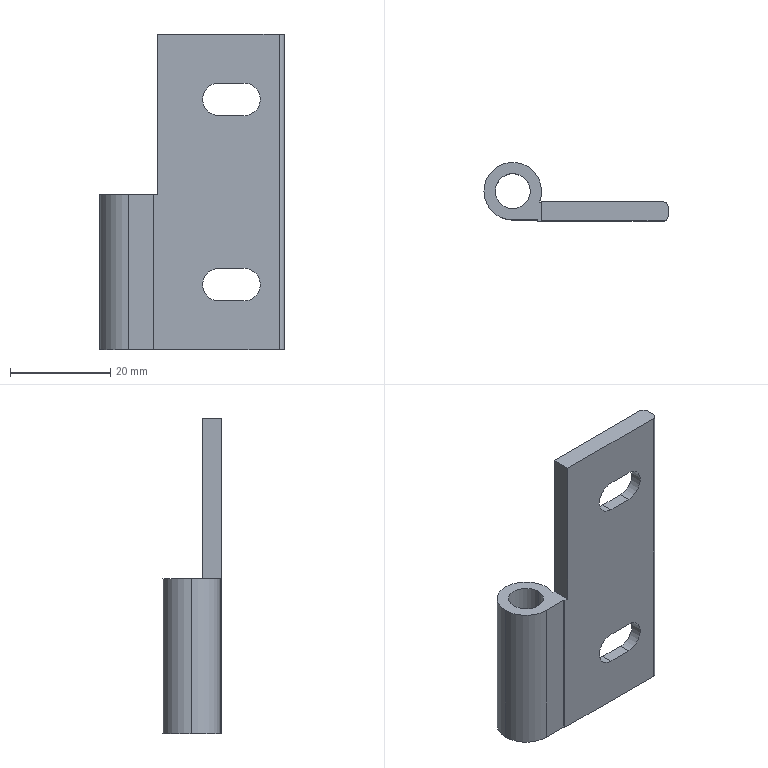Part | NX | features BREP 1 | 1 solid | 38 faces | box 36.75 x 11.75 x 63 mm | volume 7508 mm3 | cylinder 19 | plane 19 | commonest cylinder face diameters 6.5 x6 11 x6 11.5 x3 2 x2 7 x2
STEP:
#1=CARTESIAN_POINT('',(12.5,-3.7,18.5));
#2=VERTEX_POINT('',#1);
#3=CARTESIAN_POINT('',(18.,-3.7,24.));
#4=VERTEX_POINT('',#3);
#5=CARTESIAN_POINT('',(18.,-3.7,18.5));
#6=DIRECTION('',(0.,1.,0.));
#7=DIRECTION('',(-1.,0.,0.));
#8=AXIS2_PLACEMENT_3D('',#5,#6,#7);
#9=CIRCLE('',#8,5.5);
#10=EDGE_CURVE('',#2,#4,#9,.T.);
#11=ORIENTED_EDGE('',*,*,#10,.F.);
#12=CARTESIAN_POINT('',(12.5,-2.2,18.5));
#13=VERTEX_POINT('',#12);
#14=CARTESIAN_POINT('',(12.5,-3.7,18.5));
#15=DIRECTION('',(0.,1.,0.));
#16=VECTOR('',#15,1000.);
#17=LINE('',#14,#16);
#18=EDGE_CURVE('',#2,#13,#17,.T.);
#19=ORIENTED_EDGE('',*,*,#18,.T.);
#20=CARTESIAN_POINT('',(18.,-2.2,24.));
#21=VERTEX_POINT('',#20);
#22=CARTESIAN_POINT('',(18.,-2.2,18.5));
#23=DIRECTION('',(0.,1.,0.));
#24=DIRECTION('',(-1.,0.,0.));
#25=AXIS2_PLACEMENT_3D('',#22,#23,#24);
#26=CIRCLE('',#25,5.5);
#27=EDGE_CURVE('',#13,#21,#26,.T.);
#28=ORIENTED_EDGE('',*,*,#27,.T.);
#29=CARTESIAN_POINT('',(18.,-3.7,24.));
#30=DIRECTION('',(0.,1.,0.));
#31=VECTOR('',#30,1000.);
#32=LINE('',#29,#31);
#33=EDGE_CURVE('',#4,#21,#32,.T.);
#34=ORIENTED_EDGE('',*,*,#33,.F.);
#35=EDGE_LOOP('',(#11,#19,#28,#34));
#36=FACE_BOUND('',#35,.T.);
#37=CARTESIAN_POINT('',(18.,-3.7,18.5));
#38=DIRECTION('',(0.,1.,0.));
#39=DIRECTION('',(-1.,0.,0.));
#40=AXIS2_PLACEMENT_3D('',#37,#38,#39);
#41=CYLINDRICAL_SURFACE('',#40,5.5);
#42=ADVANCED_FACE('',(#36),#41,.F.);
#43=CARTESIAN_POINT('',(12.5,-3.7,-18.5));
#44=VERTEX_POINT('',#43);
#45=CARTESIAN_POINT('',(18.,-3.7,-13.));
#46=VERTEX_POINT('',#45);
#47=CARTESIAN_POINT('',(18.,-3.7,-18.5));
#48=DIRECTION('',(0.,1.,0.));
#49=DIRECTION('',(-1.,0.,0.));
#50=AXIS2_PLACEMENT_3D('',#47,#48,#49);
#51=CIRCLE('',#50,5.5);
#52=EDGE_CURVE('',#44,#46,#51,.T.);
#53=ORIENTED_EDGE('',*,*,#52,.F.);
#54=CARTESIAN_POINT('',(12.5,-2.2,-18.5));
#55=VERTEX_POINT('',#54);
#56=CARTESIAN_POINT('',(12.5,-3.7,-18.5));
#57=DIRECTION('',(0.,1.,0.));
#58=VECTOR('',#57,1000.);
#59=LINE('',#56,#58);
#60=EDGE_CURVE('',#44,#55,#59,.T.);
#61=ORIENTED_EDGE('',*,*,#60,.T.);
#62=CARTESIAN_POINT('',(18.,-2.2,-13.));
#63=VERTEX_POINT('',#62);
#64=CARTESIAN_POINT('',(18.,-2.2,-18.5));
#65=DIRECTION('',(0.,1.,0.));
#66=DIRECTION('',(-1.,0.,0.));
#67=AXIS2_PLACEMENT_3D('',#64,#65,#66);
#68=CIRCLE('',#67,5.5);
#69=EDGE_CURVE('',#55,#63,#68,.T.);
#70=ORIENTED_EDGE('',*,*,#69,.T.);
#71=CARTESIAN_POINT('',(18.,-3.7,-13.));
#72=DIRECTION('',(0.,1.,0.));
#73=VECTOR('',#72,1000.);
#74=LINE('',#71,#73);
#75=EDGE_CURVE('',#46,#63,#74,.T.);
#76=ORIENTED_EDGE('',*,*,#75,.F.);
#77=EDGE_LOOP('',(#53,#61,#70,#76));
#78=FACE_BOUND('',#77,.T.);
#79=CARTESIAN_POINT('',(18.,-3.7,-18.5));
#80=DIRECTION('',(0.,1.,0.));
#81=DIRECTION('',(-1.,0.,0.));
#82=AXIS2_PLACEMENT_3D('',#79,#80,#81);
#83=CYLINDRICAL_SURFACE('',#82,5.5);
#84=ADVANCED_FACE('',(#78),#83,.F.);
#85=CARTESIAN_POINT('',(3.5,0.,-0.5));
#86=VERTEX_POINT('',#85);
#87=CARTESIAN_POINT('',(-3.5,0.,-0.5));
#88=VERTEX_POINT('',#87);
#89=CARTESIAN_POINT('',(0.,0.,-0.5));
#90=DIRECTION('',(0.,0.,-1.));
#91=DIRECTION('',(-1.,0.,0.));
#92=AXIS2_PLACEMENT_3D('',#89,#90,#91);
#93=CIRCLE('',#92,3.5);
#94=EDGE_CURVE('',#86,#88,#93,.T.);
#95=ORIENTED_EDGE('',*,*,#94,.F.);
#96=CARTESIAN_POINT('',(3.5,0.,-31.5));
#97=VERTEX_POINT('',#96);
#98=CARTESIAN_POINT('',(3.5,0.,31.5));
#99=DIRECTION('',(0.,0.,-1.));
#100=VECTOR('',#99,1000.);
#101=LINE('',#98,#100);
#102=EDGE_CURVE('',#86,#97,#101,.T.);
#103=ORIENTED_EDGE('',*,*,#102,.T.);
#104=CARTESIAN_POINT('',(-3.5,0.,-31.5));
#105=VERTEX_POINT('',#104);
#106=CARTESIAN_POINT('',(0.,0.,-31.5));
#107=DIRECTION('',(0.,0.,1.));
#108=DIRECTION('',(1.,0.,0.));
#109=AXIS2_PLACEMENT_3D('',#106,#107,#108);
#110=CIRCLE('',#109,3.5);
#111=EDGE_CURVE('',#105,#97,#110,.T.);
#112=ORIENTED_EDGE('',*,*,#111,.F.);
#113=CARTESIAN_POINT('',(-3.5,0.,31.5));
#114=DIRECTION('',(0.,0.,-1.));
#115=VECTOR('',#114,1000.);
#116=LINE('',#113,#115);
#117=EDGE_CURVE('',#88,#105,#116,.T.);
#118=ORIENTED_EDGE('',*,*,#117,.F.);
#119=EDGE_LOOP('',(#95,#103,#112,#118));
#120=FACE_BOUND('',#119,.T.);
#121=CARTESIAN_POINT('',(0.,0.,31.5));
#122=DIRECTION('',(0.,0.,-1.));
#123=DIRECTION('',(-1.,0.,0.));
#124=AXIS2_PLACEMENT_3D('',#121,#122,#123);
#125=CYLINDRICAL_SURFACE('',#124,3.5);
#126=ADVANCED_FACE('',(#120),#125,.F.);
#127=CARTESIAN_POINT('',(-5.75,0.,-0.5));
#128=VERTEX_POINT('',#127);
#129=CARTESIAN_POINT('',(5.75,0.,-0.5));
#130=VERTEX_POINT('',#129);
#131=CARTESIAN_POINT('',(0.,0.,-0.5));
#132=DIRECTION('',(0.,0.,-1.));
#133=DIRECTION('',(-1.,0.,0.));
#134=AXIS2_PLACEMENT_3D('',#131,#132,#133);
#135=CIRCLE('',#134,5.75);
#136=EDGE_CURVE('',#128,#130,#135,.T.);
#137=ORIENTED_EDGE('',*,*,#136,.T.);
#138=CARTESIAN_POINT('',(5.75,0.,-31.5));
#139=VERTEX_POINT('',#138);
#140=CARTESIAN_POINT('',(5.75,0.,31.5));
#141=DIRECTION('',(0.,0.,-1.));
#142=VECTOR('',#141,1000.);
#143=LINE('',#140,#142);
#144=EDGE_CURVE('',#130,#139,#143,.T.);
#145=ORIENTED_EDGE('',*,*,#144,.T.);
#146=CARTESIAN_POINT('',(-5.75,0.,-31.5));
#147=VERTEX_POINT('',#146);
#148=CARTESIAN_POINT('',(0.,0.,-31.5));
#149=DIRECTION('',(0.,0.,1.));
#150=DIRECTION('',(1.,0.,0.));
#151=AXIS2_PLACEMENT_3D('',#148,#149,#150);
#152=CIRCLE('',#151,5.75);
#153=EDGE_CURVE('',#139,#147,#152,.T.);
#154=ORIENTED_EDGE('',*,*,#153,.T.);
#155=CARTESIAN_POINT('',(-5.75,0.,31.5));
#156=DIRECTION('',(0.,0.,-1.));
#157=VECTOR('',#156,1000.);
#158=LINE('',#155,#157);
#159=EDGE_CURVE('',#128,#147,#158,.T.);
#160=ORIENTED_EDGE('',*,*,#159,.F.);
#161=EDGE_LOOP('',(#137,#145,#154,#160));
#162=FACE_BOUND('',#161,.T.);
#163=CARTESIAN_POINT('',(0.,0.,31.5));
#164=DIRECTION('',(0.,0.,-1.));
#165=DIRECTION('',(-1.,0.,0.));
#166=AXIS2_PLACEMENT_3D('',#163,#164,#165);
#167=CYLINDRICAL_SURFACE('',#166,5.75);
#168=ADVANCED_FACE('',(#162),#167,.T.);
#169=CARTESIAN_POINT('',(0.,-5.75,-0.5));
#170=VERTEX_POINT('',#169);
#171=CARTESIAN_POINT('',(0.,0.,-0.5));
#172=DIRECTION('',(0.,0.,-1.));
#173=DIRECTION('',(-1.,0.,0.));
#174=AXIS2_PLACEMENT_3D('',#171,#172,#173);
#175=CIRCLE('',#174,5.75);
#176=EDGE_CURVE('',#170,#128,#175,.T.);
#177=ORIENTED_EDGE('',*,*,#176,.T.);
#178=ORIENTED_EDGE('',*,*,#159,.T.);
#179=CARTESIAN_POINT('',(0.,-5.75,-31.5));
#180=VERTEX_POINT('',#179);
#181=CARTESIAN_POINT('',(0.,0.,-31.5));
#182=DIRECTION('',(0.,0.,1.));
#183=DIRECTION('',(1.,0.,0.));
#184=AXIS2_PLACEMENT_3D('',#181,#182,#183);
#185=CIRCLE('',#184,5.75);
#186=EDGE_CURVE('',#147,#180,#185,.T.);
#187=ORIENTED_EDGE('',*,*,#186,.T.);
#188=CARTESIAN_POINT('',(0.,-5.75,31.5));
#189=DIRECTION('',(0.,0.,-1.));
#190=VECTOR('',#189,1000.);
#191=LINE('',#188,#190);
#192=EDGE_CURVE('',#170,#180,#191,.T.);
#193=ORIENTED_EDGE('',*,*,#192,.F.);
#194=EDGE_LOOP('',(#177,#178,#187,#193));
#195=FACE_BOUND('',#194,.T.);
#196=CARTESIAN_POINT('',(0.,0.,31.5));
#197=DIRECTION('',(0.,0.,-1.));
#198=DIRECTION('',(-1.,0.,0.));
#199=AXIS2_PLACEMENT_3D('',#196,#197,#198);
#200=CYLINDRICAL_SURFACE('',#199,5.75);
#201=ADVANCED_FACE('',(#195),#200,.T.);
#202=CARTESIAN_POINT('',(14.75,-6.,-18.5));
#203=VERTEX_POINT('',#202);
#204=CARTESIAN_POINT('',(18.,-6.,-15.25));
#205=VERTEX_POINT('',#204);
#206=CARTESIAN_POINT('',(18.,-6.,-18.5));
#207=DIRECTION('',(0.,1.,0.));
#208=DIRECTION('',(-1.,0.,0.));
#209=AXIS2_PLACEMENT_3D('',#206,#207,#208);
#210=CIRCLE('',#209,3.25);
#211=EDGE_CURVE('',#203,#205,#210,.T.);
#212=ORIENTED_EDGE('',*,*,#211,.F.);
#213=CARTESIAN_POINT('',(14.75,-3.7,-18.5));
#214=VERTEX_POINT('',#213);
#215=CARTESIAN_POINT('',(14.75,-6.,-18.5));
#216=DIRECTION('',(0.,1.,0.));
#217=VECTOR('',#216,1000.);
#218=LINE('',#215,#217);
#219=EDGE_CURVE('',#203,#214,#218,.T.);
#220=ORIENTED_EDGE('',*,*,#219,.T.);
#221=CARTESIAN_POINT('',(18.,-3.7,-15.25));
#222=VERTEX_POINT('',#221);
#223=CARTESIAN_POINT('',(18.,-3.7,-18.5));
#224=DIRECTION('',(0.,-1.,0.));
#225=DIRECTION('',(-1.,0.,0.));
#226=AXIS2_PLACEMENT_3D('',#223,#224,#225);
#227=CIRCLE('',#226,3.25);
#228=EDGE_CURVE('',#222,#214,#227,.T.);
#229=ORIENTED_EDGE('',*,*,#228,.F.);
#230=CARTESIAN_POINT('',(18.,-6.,-15.25));
#231=DIRECTION('',(0.,1.,0.));
#232=VECTOR('',#231,1000.);
#233=LINE('',#230,#232);
#234=EDGE_CURVE('',#205,#222,#233,.T.);
#235=ORIENTED_EDGE('',*,*,#234,.F.);
#236=EDGE_LOOP('',(#212,#220,#229,#235));
#237=FACE_BOUND('',#236,.T.);
#238=CARTESIAN_POINT('',(18.,-6.,-18.5));
#239=DIRECTION('',(0.,1.,0.));
#240=DIRECTION('',(-1.,0.,0.));
#241=AXIS2_PLACEMENT_3D('',#238,#239,#240);
#242=CYLINDRICAL_SURFACE('',#241,3.25);
#243=ADVANCED_FACE('',(#237),#242,.F.);
#244=CARTESIAN_POINT('',(14.75,-6.,18.5));
#245=VERTEX_POINT('',#244);
#246=CARTESIAN_POINT('',(18.,-6.,21.75));
#247=VERTEX_POINT('',#246);
#248=CARTESIAN_POINT('',(18.,-6.,18.5));
#249=DIRECTION('',(0.,1.,0.));
#250=DIRECTION('',(-1.,0.,0.));
#251=AXIS2_PLACEMENT_3D('',#248,#249,#250);
#252=CIRCLE('',#251,3.25);
#253=EDGE_CURVE('',#245,#247,#252,.T.);
#254=ORIENTED_EDGE('',*,*,#253,.F.);
#255=CARTESIAN_POINT('',(14.75,-3.7,18.5));
#256=VERTEX_POINT('',#255);
#257=CARTESIAN_POINT('',(14.75,-6.,18.5));
#258=DIRECTION('',(0.,1.,0.));
#259=VECTOR('',#258,1000.);
#260=LINE('',#257,#259);
#261=EDGE_CURVE('',#245,#256,#260,.T.);
#262=ORIENTED_EDGE('',*,*,#261,.T.);
#263=CARTESIAN_POINT('',(18.,-3.7,21.75));
#264=VERTEX_POINT('',#263);
#265=CARTESIAN_POINT('',(18.,-3.7,18.5));
#266=DIRECTION('',(0.,-1.,0.));
#267=DIRECTION('',(-1.,0.,0.));
#268=AXIS2_PLACEMENT_3D('',#265,#266,#267);
#269=CIRCLE('',#268,3.25);
#270=EDGE_CURVE('',#264,#256,#269,.T.);
#271=ORIENTED_EDGE('',*,*,#270,.F.);
#272=CARTESIAN_POINT('',(18.,-6.,21.75));
#273=DIRECTION('',(0.,1.,0.));
#274=VECTOR('',#273,1000.);
#275=LINE('',#272,#274);
#276=EDGE_CURVE('',#247,#264,#275,.T.);
#277=ORIENTED_EDGE('',*,*,#276,.F.);
#278=EDGE_LOOP('',(#254,#262,#271,#277));
#279=FACE_BOUND('',#278,.T.);
#280=CARTESIAN_POINT('',(18.,-6.,18.5));
#281=DIRECTION('',(0.,1.,0.));
#282=DIRECTION('',(-1.,0.,0.));
#283=AXIS2_PLACEMENT_3D('',#280,#281,#282);
#284=CYLINDRICAL_SURFACE('',#283,3.25);
#285=ADVANCED_FACE('',(#279),#284,.F.);
#286=ORIENTED_EDGE('',*,*,#261,.F.);
#287=CARTESIAN_POINT('',(18.,-6.,15.25));
#288=VERTEX_POINT('',#287);
#289=CARTESIAN_POINT('',(18.,-6.,18.5));
#290=DIRECTION('',(0.,1.,0.));
#291=DIRECTION('',(-1.,0.,0.));
#292=AXIS2_PLACEMENT_3D('',#289,#290,#291);
#293=CIRCLE('',#292,3.25);
#294=EDGE_CURVE('',#288,#245,#293,.T.);
#295=ORIENTED_EDGE('',*,*,#294,.F.);
#296=CARTESIAN_POINT('',(18.,-3.7,15.25));
#297=VERTEX_POINT('',#296);
#298=CARTESIAN_POINT('',(18.,-6.,15.25));
#299=DIRECTION('',(0.,1.,0.));
#300=VECTOR('',#299,1000.);
#301=LINE('',#298,#300);
#302=EDGE_CURVE('',#288,#297,#301,.T.);
#303=ORIENTED_EDGE('',*,*,#302,.T.);
#304=CARTESIAN_POINT('',(18.,-3.7,18.5));
#305=DIRECTION('',(0.,-1.,0.));
#306=DIRECTION('',(-1.,0.,0.));
#307=AXIS2_PLACEMENT_3D('',#304,#305,#306);
#308=CIRCLE('',#307,3.25);
#309=EDGE_CURVE('',#256,#297,#308,.T.);
#310=ORIENTED_EDGE('',*,*,#309,.F.);
#311=EDGE_LOOP('',(#286,#295,#303,#310));
#312=FACE_BOUND('',#311,.T.);
#313=CARTESIAN_POINT('',(18.,-6.,18.5));
#314=DIRECTION('',(0.,1.,0.));
#315=DIRECTION('',(-1.,0.,0.));
#316=AXIS2_PLACEMENT_3D('',#313,#314,#315);
#317=CYLINDRICAL_SURFACE('',#316,3.25);
#318=ADVANCED_FACE('',(#312),#317,.F.);
#319=CARTESIAN_POINT('',(23.,-3.7,15.25));
#320=VERTEX_POINT('',#319);
#321=CARTESIAN_POINT('',(18.,-3.7,15.25));
#322=DIRECTION('',(1.,0.,0.));
#323=VECTOR('',#322,1000.);
#324=LINE('',#321,#323);
#325=EDGE_CURVE('',#297,#320,#324,.T.);
#326=ORIENTED_EDGE('',*,*,#325,.F.);
#327=ORIENTED_EDGE('',*,*,#302,.F.);
#328=CARTESIAN_POINT('',(23.,-6.,15.25));
#329=VERTEX_POINT('',#328);
#330=CARTESIAN_POINT('',(18.,-6.,15.25));
#331=DIRECTION('',(-1.,0.,0.));
#332=VECTOR('',#331,1000.);
#333=LINE('',#330,#332);
#334=EDGE_CURVE('',#329,#288,#333,.T.);
#335=ORIENTED_EDGE('',*,*,#334,.F.);
#336=CARTESIAN_POINT('',(23.,-6.,15.25));
#337=DIRECTION('',(0.,1.,0.));
#338=VECTOR('',#337,1000.);
#339=LINE('',#336,#338);
#340=EDGE_CURVE('',#329,#320,#339,.T.);
#341=ORIENTED_EDGE('',*,*,#340,.T.);
#342=EDGE_LOOP('',(#326,#327,#335,#341));
#343=FACE_BOUND('',#342,.T.);
#344=CARTESIAN_POINT('',(18.,-6.,15.25));
#345=DIRECTION('',(0.,0.,-1.));
#346=DIRECTION('',(0.,-1.,0.));
#347=AXIS2_PLACEMENT_3D('',#344,#345,#346);
#348=PLANE('',#347);
#349=ADVANCED_FACE('',(#343),#348,.F.);
#350=CARTESIAN_POINT('',(23.,-3.7,21.75));
#351=VERTEX_POINT('',#350);
#352=CARTESIAN_POINT('',(23.,-3.7,18.5));
#353=DIRECTION('',(0.,-1.,0.));
#354=DIRECTION('',(-1.,0.,0.));
#355=AXIS2_PLACEMENT_3D('',#352,#353,#354);
#356=CIRCLE('',#355,3.25);
#357=EDGE_CURVE('',#320,#351,#356,.T.);
#358=ORIENTED_EDGE('',*,*,#357,.F.);
#359=ORIENTED_EDGE('',*,*,#340,.F.);
#360=CARTESIAN_POINT('',(23.,-6.,21.75));
#361=VERTEX_POINT('',#360);
#362=CARTESIAN_POINT('',(23.,-6.,18.5));
#363=DIRECTION('',(0.,1.,0.));
#364=DIRECTION('',(-1.,0.,0.));
#365=AXIS2_PLACEMENT_3D('',#362,#363,#364);
#366=CIRCLE('',#365,3.25);
#367=EDGE_CURVE('',#361,#329,#366,.T.);
#368=ORIENTED_EDGE('',*,*,#367,.F.);
#369=CARTESIAN_POINT('',(23.,-6.,21.75));
#370=DIRECTION('',(0.,1.,0.));
#371=VECTOR('',#370,1000.);
#372=LINE('',#369,#371);
#373=EDGE_CURVE('',#361,#351,#372,.T.);
#374=ORIENTED_EDGE('',*,*,#373,.T.);
#375=EDGE_LOOP('',(#358,#359,#368,#374));
#376=FACE_BOUND('',#375,.T.);
#377=CARTESIAN_POINT('',(23.,-6.,18.5));
#378=DIRECTION('',(0.,1.,0.));
#379=DIRECTION('',(-1.,0.,0.));
#380=AXIS2_PLACEMENT_3D('',#377,#378,#379);
#381=CYLINDRICAL_SURFACE('',#380,3.25);
#382=ADVANCED_FACE('',(#376),#381,.F.);
#383=CARTESIAN_POINT('',(18.,-3.7,21.75));
#384=DIRECTION('',(-1.,0.,0.));
#385=VECTOR('',#384,1000.);
#386=LINE('',#383,#385);
#387=EDGE_CURVE('',#351,#264,#386,.T.);
#388=ORIENTED_EDGE('',*,*,#387,.F.);
#389=ORIENTED_EDGE('',*,*,#373,.F.);
#390=CARTESIAN_POINT('',(18.,-6.,21.75));
#391=DIRECTION('',(1.,0.,0.));
#392=VECTOR('',#391,1000.);
#393=LINE('',#390,#392);
#394=EDGE_CURVE('',#247,#361,#393,.T.);
#395=ORIENTED_EDGE('',*,*,#394,.F.);
#396=ORIENTED_EDGE('',*,*,#276,.T.);
#397=EDGE_LOOP('',(#388,#389,#395,#396));
#398=FACE_BOUND('',#397,.T.);
#399=CARTESIAN_POINT('',(18.,-6.,21.75));
#400=DIRECTION('',(0.,0.,1.));
#401=DIRECTION('',(1.,0.,0.));
#402=AXIS2_PLACEMENT_3D('',#399,#400,#401);
#403=PLANE('',#402);
#404=ADVANCED_FACE('',(#398),#403,.F.);
#405=ORIENTED_EDGE('',*,*,#219,.F.);
#406=CARTESIAN_POINT('',(18.,-6.,-21.75));
#407=VERTEX_POINT('',#406);
#408=CARTESIAN_POINT('',(18.,-6.,-18.5));
#409=DIRECTION('',(0.,1.,0.));
#410=DIRECTION('',(-1.,0.,0.));
#411=AXIS2_PLACEMENT_3D('',#408,#409,#410);
#412=CIRCLE('',#411,3.25);
#413=EDGE_CURVE('',#407,#203,#412,.T.);
#414=ORIENTED_EDGE('',*,*,#413,.F.);
#415=CARTESIAN_POINT('',(18.,-3.7,-21.75));
#416=VERTEX_POINT('',#415);
#417=CARTESIAN_POINT('',(18.,-6.,-21.75));
#418=DIRECTION('',(0.,1.,0.));
#419=VECTOR('',#418,1000.);
#420=LINE('',#417,#419);
#421=EDGE_CURVE('',#407,#416,#420,.T.);
#422=ORIENTED_EDGE('',*,*,#421,.T.);
#423=CARTESIAN_POINT('',(18.,-3.7,-18.5));
#424=DIRECTION('',(0.,-1.,0.));
#425=DIRECTION('',(-1.,0.,0.));
#426=AXIS2_PLACEMENT_3D('',#423,#424,#425);
#427=CIRCLE('',#426,3.25);
#428=EDGE_CURVE('',#214,#416,#427,.T.);
#429=ORIENTED_EDGE('',*,*,#428,.F.);
#430=EDGE_LOOP('',(#405,#414,#422,#429));
#431=FACE_BOUND('',#430,.T.);
#432=CARTESIAN_POINT('',(18.,-6.,-18.5));
#433=DIRECTION('',(0.,1.,0.));
#434=DIRECTION('',(-1.,0.,0.));
#435=AXIS2_PLACEMENT_3D('',#432,#433,#434);
#436=CYLINDRICAL_SURFACE('',#435,3.25);
#437=ADVANCED_FACE('',(#431),#436,.F.);
#438=CARTESIAN_POINT('',(23.,-3.7,-21.75));
#439=VERTEX_POINT('',#438);
#440=CARTESIAN_POINT('',(18.,-3.7,-21.75));
#441=DIRECTION('',(1.,0.,0.));
#442=VECTOR('',#441,1000.);
#443=LINE('',#440,#442);
#444=EDGE_CURVE('',#416,#439,#443,.T.);
#445=ORIENTED_EDGE('',*,*,#444,.F.);
#446=ORIENTED_EDGE('',*,*,#421,.F.);
#447=CARTESIAN_POINT('',(23.,-6.,-21.75));
#448=VERTEX_POINT('',#447);
#449=CARTESIAN_POINT('',(18.,-6.,-21.75));
#450=DIRECTION('',(-1.,0.,0.));
#451=VECTOR('',#450,1000.);
#452=LINE('',#449,#451);
#453=EDGE_CURVE('',#448,#407,#452,.T.);
#454=ORIENTED_EDGE('',*,*,#453,.F.);
#455=CARTESIAN_POINT('',(23.,-6.,-21.75));
#456=DIRECTION('',(0.,1.,0.));
#457=VECTOR('',#456,1000.);
#458=LINE('',#455,#457);
#459=EDGE_CURVE('',#448,#439,#458,.T.);
#460=ORIENTED_EDGE('',*,*,#459,.T.);
#461=EDGE_LOOP('',(#445,#446,#454,#460));
#462=FACE_BOUND('',#461,.T.);
#463=CARTESIAN_POINT('',(18.,-6.,-21.75));
#464=DIRECTION('',(0.,0.,-1.));
#465=DIRECTION('',(0.,-1.,0.));
#466=AXIS2_PLACEMENT_3D('',#463,#464,#465);
#467=PLANE('',#466);
#468=ADVANCED_FACE('',(#462),#467,.F.);
#469=CARTESIAN_POINT('',(23.,-3.7,-15.25));
#470=VERTEX_POINT('',#469);
#471=CARTESIAN_POINT('',(23.,-3.7,-18.5));
#472=DIRECTION('',(0.,-1.,0.));
#473=DIRECTION('',(-1.,0.,0.));
#474=AXIS2_PLACEMENT_3D('',#471,#472,#473);
#475=CIRCLE('',#474,3.25);
#476=EDGE_CURVE('',#439,#470,#475,.T.);
#477=ORIENTED_EDGE('',*,*,#476,.F.);
#478=ORIENTED_EDGE('',*,*,#459,.F.);
#479=CARTESIAN_POINT('',(23.,-6.,-15.25));
#480=VERTEX_POINT('',#479);
#481=CARTESIAN_POINT('',(23.,-6.,-18.5));
#482=DIRECTION('',(0.,1.,0.));
#483=DIRECTION('',(-1.,0.,0.));
#484=AXIS2_PLACEMENT_3D('',#481,#482,#483);
#485=CIRCLE('',#484,3.25);
#486=EDGE_CURVE('',#480,#448,#485,.T.);
#487=ORIENTED_EDGE('',*,*,#486,.F.);
#488=CARTESIAN_POINT('',(23.,-6.,-15.25));
#489=DIRECTION('',(0.,1.,0.));
#490=VECTOR('',#489,1000.);
#491=LINE('',#488,#490);
#492=EDGE_CURVE('',#480,#470,#491,.T.);
#493=ORIENTED_EDGE('',*,*,#492,.T.);
#494=EDGE_LOOP('',(#477,#478,#487,#493));
#495=FACE_BOUND('',#494,.T.);
#496=CARTESIAN_POINT('',(23.,-6.,-18.5));
#497=DIRECTION('',(0.,1.,0.));
#498=DIRECTION('',(-1.,0.,0.));
#499=AXIS2_PLACEMENT_3D('',#496,#497,#498);
#500=CYLINDRICAL_SURFACE('',#499,3.25);
#501=ADVANCED_FACE('',(#495),#500,.F.);
#502=CARTESIAN_POINT('',(18.,-3.7,-15.25));
#503=DIRECTION('',(-1.,0.,0.));
#504=VECTOR('',#503,1000.);
#505=LINE('',#502,#504);
#506=EDGE_CURVE('',#470,#222,#505,.T.);
#507=ORIENTED_EDGE('',*,*,#506,.F.);
#508=ORIENTED_EDGE('',*,*,#492,.F.);
#509=CARTESIAN_POINT('',(18.,-6.,-15.25));
#510=DIRECTION('',(1.,0.,0.));
#511=VECTOR('',#510,1000.);
#512=LINE('',#509,#511);
#513=EDGE_CURVE('',#205,#480,#512,.T.);
#514=ORIENTED_EDGE('',*,*,#513,.F.);
#515=ORIENTED_EDGE('',*,*,#234,.T.);
#516=EDGE_LOOP('',(#507,#508,#514,#515));
#517=FACE_BOUND('',#516,.T.);
#518=CARTESIAN_POINT('',(18.,-6.,-15.25));
#519=DIRECTION('',(0.,0.,1.));
#520=DIRECTION('',(1.,0.,0.));
#521=AXIS2_PLACEMENT_3D('',#518,#519,#520);
#522=PLANE('',#521);
#523=ADVANCED_FACE('',(#517),#522,.F.);
#524=ORIENTED_EDGE('',*,*,#144,.F.);
#525=CARTESIAN_POINT('',(5.312,-2.2,-0.5));
#526=VERTEX_POINT('',#525);
#527=CARTESIAN_POINT('',(0.,0.,-0.5));
#528=DIRECTION('',(0.,0.,-1.));
#529=DIRECTION('',(-1.,0.,0.));
#530=AXIS2_PLACEMENT_3D('',#527,#528,#529);
#531=CIRCLE('',#530,5.75);
#532=EDGE_CURVE('',#130,#526,#531,.T.);
#533=ORIENTED_EDGE('',*,*,#532,.T.);
#534=CARTESIAN_POINT('',(5.312,-2.2,-31.5));
#535=VERTEX_POINT('',#534);
#536=CARTESIAN_POINT('',(5.312,-2.2,31.5));
#537=DIRECTION('',(0.,0.,-1.));
#538=VECTOR('',#537,1000.);
#539=LINE('',#536,#538);
#540=EDGE_CURVE('',#526,#535,#539,.T.);
#541=ORIENTED_EDGE('',*,*,#540,.T.);
#542=CARTESIAN_POINT('',(0.,0.,-31.5));
#543=DIRECTION('',(0.,0.,1.));
#544=DIRECTION('',(1.,0.,0.));
#545=AXIS2_PLACEMENT_3D('',#542,#543,#544);
#546=CIRCLE('',#545,5.75);
#547=EDGE_CURVE('',#535,#139,#546,.T.);
#548=ORIENTED_EDGE('',*,*,#547,.T.);
#549=EDGE_LOOP('',(#524,#533,#541,#548));
#550=FACE_BOUND('',#549,.T.);
#551=CARTESIAN_POINT('',(0.,0.,31.5));
#552=DIRECTION('',(0.,0.,-1.));
#553=DIRECTION('',(-1.,0.,0.));
#554=AXIS2_PLACEMENT_3D('',#551,#552,#553);
#555=CYLINDRICAL_SURFACE('',#554,5.75);
#556=ADVANCED_FACE('',(#550),#555,.T.);
#557=CARTESIAN_POINT('',(5.75,-2.2,31.5));
#558=VERTEX_POINT('',#557);
#559=CARTESIAN_POINT('',(5.75,-6.,31.5));
#560=VERTEX_POINT('',#559);
#561=CARTESIAN_POINT('',(5.75,5.75,31.5));
#562=DIRECTION('',(0.,-1.,0.));
#563=VECTOR('',#562,1000.);
#564=LINE('',#561,#563);
#565=EDGE_CURVE('',#558,#560,#564,.T.);
#566=ORIENTED_EDGE('',*,*,#565,.T.);
#567=CARTESIAN_POINT('',(30.,-6.,31.5));
#568=VERTEX_POINT('',#567);
#569=CARTESIAN_POINT('',(5.,-6.,31.5));
#570=DIRECTION('',(1.,0.,0.));
#571=VECTOR('',#570,1000.);
#572=LINE('',#569,#571);
#573=EDGE_CURVE('',#560,#568,#572,.T.);
#574=ORIENTED_EDGE('',*,*,#573,.T.);
#575=CARTESIAN_POINT('',(31.,-5.,31.5));
#576=VERTEX_POINT('',#575);
#577=CARTESIAN_POINT('',(30.,-5.,31.5));
#578=DIRECTION('',(0.,0.,1.));
#579=DIRECTION('',(1.,0.,0.));
#580=AXIS2_PLACEMENT_3D('',#577,#578,#579);
#581=CIRCLE('',#580,1.);
#582=EDGE_CURVE('',#568,#576,#581,.T.);
#583=ORIENTED_EDGE('',*,*,#582,.T.);
#584=CARTESIAN_POINT('',(31.,-3.2,31.5));
#585=VERTEX_POINT('',#584);
#586=CARTESIAN_POINT('',(31.,-6.,31.5));
#587=DIRECTION('',(0.,1.,0.));
#588=VECTOR('',#587,1000.);
#589=LINE('',#586,#588);
#590=EDGE_CURVE('',#576,#585,#589,.T.);
#591=ORIENTED_EDGE('',*,*,#590,.T.);
#592=CARTESIAN_POINT('',(30.,-2.2,31.5));
#593=VERTEX_POINT('',#592);
#594=CARTESIAN_POINT('',(30.,-3.2,31.5));
#595=DIRECTION('',(0.,0.,1.));
#596=DIRECTION('',(1.,0.,0.));
#597=AXIS2_PLACEMENT_3D('',#594,#595,#596);
#598=CIRCLE('',#597,1.);
#599=EDGE_CURVE('',#585,#593,#598,.T.);
#600=ORIENTED_EDGE('',*,*,#599,.T.);
#601=CARTESIAN_POINT('',(31.,-2.2,31.5));
#602=DIRECTION('',(-1.,0.,0.));
#603=VECTOR('',#602,1000.);
#604=LINE('',#601,#603);
#605=EDGE_CURVE('',#593,#558,#604,.T.);
#606=ORIENTED_EDGE('',*,*,#605,.T.);
#607=EDGE_LOOP('',(#566,#574,#583,#591,#600,#606));
#608=FACE_BOUND('',#607,.T.);
#609=CARTESIAN_POINT('',(0.,0.,31.5));
#610=DIRECTION('',(0.,0.,1.));
#611=DIRECTION('',(1.,0.,0.));
#612=AXIS2_PLACEMENT_3D('',#609,#610,#611);
#613=PLANE('',#612);
#614=ADVANCED_FACE('',(#608),#613,.T.);
#615=CARTESIAN_POINT('',(31.,-5.,-31.5));
#616=VERTEX_POINT('',#615);
#617=CARTESIAN_POINT('',(31.,-3.2,-31.5));
#618=VERTEX_POINT('',#617);
#619=CARTESIAN_POINT('',(31.,-6.,-31.5));
#620=DIRECTION('',(0.,1.,0.));
#621=VECTOR('',#620,1000.);
#622=LINE('',#619,#621);
#623=EDGE_CURVE('',#616,#618,#622,.T.);
#624=ORIENTED_EDGE('',*,*,#623,.F.);
#625=CARTESIAN_POINT('',(30.,-6.,-31.5));
#626=VERTEX_POINT('',#625);
#627=CARTESIAN_POINT('',(30.,-5.,-31.5));
#628=DIRECTION('',(0.,0.,-1.));
#629=DIRECTION('',(1.,0.,0.));
#630=AXIS2_PLACEMENT_3D('',#627,#628,#629);
#631=CIRCLE('',#630,1.);
#632=EDGE_CURVE('',#616,#626,#631,.T.);
#633=ORIENTED_EDGE('',*,*,#632,.T.);
#634=CARTESIAN_POINT('',(5.,-6.,-31.5));
#635=VERTEX_POINT('',#634);
#636=CARTESIAN_POINT('',(5.,-6.,-31.5));
#637=DIRECTION('',(1.,0.,0.));
#638=VECTOR('',#637,1000.);
#639=LINE('',#636,#638);
#640=EDGE_CURVE('',#635,#626,#639,.T.);
#641=ORIENTED_EDGE('',*,*,#640,.F.);
#642=CARTESIAN_POINT('',(5.,-5.75,-31.5));
#643=VERTEX_POINT('',#642);
#644=CARTESIAN_POINT('',(5.,-5.75,-31.5));
#645=DIRECTION('',(0.,-1.,0.));
#646=VECTOR('',#645,1000.);
#647=LINE('',#644,#646);
#648=EDGE_CURVE('',#643,#635,#647,.T.);
#649=ORIENTED_EDGE('',*,*,#648,.F.);
#650=CARTESIAN_POINT('',(0.,-5.75,-31.5));
#651=DIRECTION('',(1.,0.,0.));
#652=VECTOR('',#651,1000.);
#653=LINE('',#650,#652);
#654=EDGE_CURVE('',#180,#643,#653,.T.);
#655=ORIENTED_EDGE('',*,*,#654,.F.);
#656=ORIENTED_EDGE('',*,*,#186,.F.);
#657=ORIENTED_EDGE('',*,*,#153,.F.);
#658=ORIENTED_EDGE('',*,*,#547,.F.);
#659=CARTESIAN_POINT('',(30.,-2.2,-31.5));
#660=VERTEX_POINT('',#659);
#661=CARTESIAN_POINT('',(31.,-2.2,-31.5));
#662=DIRECTION('',(-1.,0.,0.));
#663=VECTOR('',#662,1000.);
#664=LINE('',#661,#663);
#665=EDGE_CURVE('',#660,#535,#664,.T.);
#666=ORIENTED_EDGE('',*,*,#665,.F.);
#667=CARTESIAN_POINT('',(30.,-3.2,-31.5));
#668=DIRECTION('',(0.,0.,-1.));
#669=DIRECTION('',(1.,0.,0.));
#670=AXIS2_PLACEMENT_3D('',#667,#668,#669);
#671=CIRCLE('',#670,1.);
#672=EDGE_CURVE('',#660,#618,#671,.T.);
#673=ORIENTED_EDGE('',*,*,#672,.T.);
#674=EDGE_LOOP('',(#624,#633,#641,#649,#655,#656,#657,#658,#666,#673));
#675=FACE_BOUND('',#674,.T.);
#676=ORIENTED_EDGE('',*,*,#111,.T.);
#677=CARTESIAN_POINT('',(0.,0.,-31.5));
#678=DIRECTION('',(0.,0.,1.));
#679=DIRECTION('',(1.,0.,0.));
#680=AXIS2_PLACEMENT_3D('',#677,#678,#679);
#681=CIRCLE('',#680,3.5);
#682=EDGE_CURVE('',#97,#105,#681,.T.);
#683=ORIENTED_EDGE('',*,*,#682,.T.);
#684=EDGE_LOOP('',(#676,#683));
#685=FACE_BOUND('',#684,.T.);
#686=CARTESIAN_POINT('',(0.,0.,-31.5));
#687=DIRECTION('',(0.,0.,1.));
#688=DIRECTION('',(1.,0.,0.));
#689=AXIS2_PLACEMENT_3D('',#686,#687,#688);
#690=PLANE('',#689);
#691=ADVANCED_FACE('',(#675,#685),#690,.F.);
#692=CARTESIAN_POINT('',(5.,-5.75,-0.5));
#693=VERTEX_POINT('',#692);
#694=CARTESIAN_POINT('',(5.,-5.75,31.5));
#695=DIRECTION('',(0.,0.,-1.));
#696=VECTOR('',#695,1000.);
#697=LINE('',#694,#696);
#698=EDGE_CURVE('',#693,#643,#697,.T.);
#699=ORIENTED_EDGE('',*,*,#698,.F.);
#700=CARTESIAN_POINT('',(0.,-5.75,-0.5));
#701=DIRECTION('',(-1.,0.,0.));
#702=VECTOR('',#701,1000.);
#703=LINE('',#700,#702);
#704=EDGE_CURVE('',#693,#170,#703,.T.);
#705=ORIENTED_EDGE('',*,*,#704,.T.);
#706=ORIENTED_EDGE('',*,*,#192,.T.);
#707=ORIENTED_EDGE('',*,*,#654,.T.);
#708=EDGE_LOOP('',(#699,#705,#706,#707));
#709=FACE_BOUND('',#708,.T.);
#710=CARTESIAN_POINT('',(0.,-5.75,31.5));
#711=DIRECTION('',(0.,1.,0.));
#712=DIRECTION('',(1.,0.,0.));
#713=AXIS2_PLACEMENT_3D('',#710,#711,#712);
#714=PLANE('',#713);
#715=ADVANCED_FACE('',(#709),#714,.F.);
#716=CARTESIAN_POINT('',(5.,-6.,-0.5));
#717=VERTEX_POINT('',#716);
#718=CARTESIAN_POINT('',(5.,-6.,31.5));
#719=DIRECTION('',(0.,0.,-1.));
#720=VECTOR('',#719,1000.);
#721=LINE('',#718,#720);
#722=EDGE_CURVE('',#717,#635,#721,.T.);
#723=ORIENTED_EDGE('',*,*,#722,.F.);
#724=CARTESIAN_POINT('',(5.,-5.75,-0.5));
#725=DIRECTION('',(0.,1.,0.));
#726=VECTOR('',#725,1000.);
#727=LINE('',#724,#726);
#728=EDGE_CURVE('',#717,#693,#727,.T.);
#729=ORIENTED_EDGE('',*,*,#728,.T.);
#730=ORIENTED_EDGE('',*,*,#698,.T.);
#731=ORIENTED_EDGE('',*,*,#648,.T.);
#732=EDGE_LOOP('',(#723,#729,#730,#731));
#733=FACE_BOUND('',#732,.T.);
#734=CARTESIAN_POINT('',(5.,-5.75,31.5));
#735=DIRECTION('',(1.,0.,0.));
#736=DIRECTION('',(0.,1.,0.));
#737=AXIS2_PLACEMENT_3D('',#734,#735,#736);
#738=PLANE('',#737);
#739=ADVANCED_FACE('',(#733),#738,.F.);
#740=ORIENTED_EDGE('',*,*,#573,.F.);
#741=CARTESIAN_POINT('',(5.75,-6.,-0.5));
#742=VERTEX_POINT('',#741);
#743=CARTESIAN_POINT('',(5.75,-6.,-0.5));
#744=DIRECTION('',(0.,0.,1.));
#745=VECTOR('',#744,1000.);
#746=LINE('',#743,#745);
#747=EDGE_CURVE('',#742,#560,#746,.T.);
#748=ORIENTED_EDGE('',*,*,#747,.F.);
#749=CARTESIAN_POINT('',(-5.75,-6.,-0.5));
#750=DIRECTION('',(1.,0.,0.));
#751=VECTOR('',#750,1000.);
#752=LINE('',#749,#751);
#753=EDGE_CURVE('',#717,#742,#752,.T.);
#754=ORIENTED_EDGE('',*,*,#753,.F.);
#755=ORIENTED_EDGE('',*,*,#722,.T.);
#756=ORIENTED_EDGE('',*,*,#640,.T.);
#757=CARTESIAN_POINT('',(30.,-6.,31.5));
#758=DIRECTION('',(0.,0.,1.));
#759=VECTOR('',#758,1000.);
#760=LINE('',#757,#759);
#761=EDGE_CURVE('',#626,#568,#760,.T.);
#762=ORIENTED_EDGE('',*,*,#761,.T.);
#763=EDGE_LOOP('',(#740,#748,#754,#755,#756,#762));
#764=FACE_BOUND('',#763,.T.);
#765=ORIENTED_EDGE('',*,*,#334,.T.);
#766=ORIENTED_EDGE('',*,*,#294,.T.);
#767=ORIENTED_EDGE('',*,*,#253,.T.);
#768=ORIENTED_EDGE('',*,*,#394,.T.);
#769=ORIENTED_EDGE('',*,*,#367,.T.);
#770=EDGE_LOOP('',(#765,#766,#767,#768,#769));
#771=FACE_BOUND('',#770,.T.);
#772=ORIENTED_EDGE('',*,*,#453,.T.);
#773=ORIENTED_EDGE('',*,*,#413,.T.);
#774=ORIENTED_EDGE('',*,*,#211,.T.);
#775=ORIENTED_EDGE('',*,*,#513,.T.);
#776=ORIENTED_EDGE('',*,*,#486,.T.);
#777=EDGE_LOOP('',(#772,#773,#774,#775,#776));
#778=FACE_BOUND('',#777,.T.);
#779=CARTESIAN_POINT('',(5.,-6.,31.5));
#780=DIRECTION('',(0.,1.,0.));
#781=DIRECTION('',(1.,0.,0.));
#782=AXIS2_PLACEMENT_3D('',#779,#780,#781);
#783=PLANE('',#782);
#784=ADVANCED_FACE('',(#764,#771,#778),#783,.F.);
#785=ORIENTED_EDGE('',*,*,#590,.F.);
#786=CARTESIAN_POINT('',(31.,-5.,31.5));
#787=DIRECTION('',(0.,0.,-1.));
#788=VECTOR('',#787,1000.);
#789=LINE('',#786,#788);
#790=EDGE_CURVE('',#576,#616,#789,.T.);
#791=ORIENTED_EDGE('',*,*,#790,.T.);
#792=ORIENTED_EDGE('',*,*,#623,.T.);
#793=CARTESIAN_POINT('',(31.,-3.2,31.5));
#794=DIRECTION('',(0.,0.,1.));
#795=VECTOR('',#794,1000.);
#796=LINE('',#793,#795);
#797=EDGE_CURVE('',#618,#585,#796,.T.);
#798=ORIENTED_EDGE('',*,*,#797,.T.);
#799=EDGE_LOOP('',(#785,#791,#792,#798));
#800=FACE_BOUND('',#799,.T.);
#801=CARTESIAN_POINT('',(31.,-6.,31.5));
#802=DIRECTION('',(-1.,0.,0.));
#803=DIRECTION('',(0.,0.,1.));
#804=AXIS2_PLACEMENT_3D('',#801,#802,#803);
#805=PLANE('',#804);
#806=ADVANCED_FACE('',(#800),#805,.F.);
#807=CARTESIAN_POINT('',(5.75,-2.2,-0.5));
#808=VERTEX_POINT('',#807);
#809=CARTESIAN_POINT('',(31.,-2.2,-0.5));
#810=DIRECTION('',(1.,0.,0.));
#811=VECTOR('',#810,1000.);
#812=LINE('',#809,#811);
#813=EDGE_CURVE('',#526,#808,#812,.T.);
#814=ORIENTED_EDGE('',*,*,#813,.T.);
#815=CARTESIAN_POINT('',(5.75,-2.2,31.5));
#816=DIRECTION('',(0.,0.,1.));
#817=VECTOR('',#816,1000.);
#818=LINE('',#815,#817);
#819=EDGE_CURVE('',#808,#558,#818,.T.);
#820=ORIENTED_EDGE('',*,*,#819,.T.);
#821=ORIENTED_EDGE('',*,*,#605,.F.);
#822=CARTESIAN_POINT('',(30.,-2.2,31.5));
#823=DIRECTION('',(0.,0.,-1.));
#824=VECTOR('',#823,1000.);
#825=LINE('',#822,#824);
#826=EDGE_CURVE('',#593,#660,#825,.T.);
#827=ORIENTED_EDGE('',*,*,#826,.T.);
#828=ORIENTED_EDGE('',*,*,#665,.T.);
#829=ORIENTED_EDGE('',*,*,#540,.F.);
#830=EDGE_LOOP('',(#814,#820,#821,#827,#828,#829));
#831=FACE_BOUND('',#830,.T.);
#832=CARTESIAN_POINT('',(23.,-2.2,24.));
#833=VERTEX_POINT('',#832);
#834=CARTESIAN_POINT('',(18.,-2.2,24.));
#835=DIRECTION('',(1.,0.,0.));
#836=VECTOR('',#835,1000.);
#837=LINE('',#834,#836);
#838=EDGE_CURVE('',#21,#833,#837,.T.);
#839=ORIENTED_EDGE('',*,*,#838,.F.);
#840=ORIENTED_EDGE('',*,*,#27,.F.);
#841=CARTESIAN_POINT('',(18.,-2.2,13.));
#842=VERTEX_POINT('',#841);
#843=CARTESIAN_POINT('',(18.,-2.2,18.5));
#844=DIRECTION('',(0.,1.,0.));
#845=DIRECTION('',(-1.,0.,0.));
#846=AXIS2_PLACEMENT_3D('',#843,#844,#845);
#847=CIRCLE('',#846,5.5);
#848=EDGE_CURVE('',#842,#13,#847,.T.);
#849=ORIENTED_EDGE('',*,*,#848,.F.);
#850=CARTESIAN_POINT('',(23.,-2.2,13.));
#851=VERTEX_POINT('',#850);
#852=CARTESIAN_POINT('',(18.,-2.2,13.));
#853=DIRECTION('',(-1.,0.,0.));
#854=VECTOR('',#853,1000.);
#855=LINE('',#852,#854);
#856=EDGE_CURVE('',#851,#842,#855,.T.);
#857=ORIENTED_EDGE('',*,*,#856,.F.);
#858=CARTESIAN_POINT('',(23.,-2.2,18.5));
#859=DIRECTION('',(0.,1.,0.));
#860=DIRECTION('',(-1.,0.,0.));
#861=AXIS2_PLACEMENT_3D('',#858,#859,#860);
#862=CIRCLE('',#861,5.5);
#863=EDGE_CURVE('',#833,#851,#862,.T.);
#864=ORIENTED_EDGE('',*,*,#863,.F.);
#865=EDGE_LOOP('',(#839,#840,#849,#857,#864));
#866=FACE_BOUND('',#865,.T.);
#867=CARTESIAN_POINT('',(23.,-2.2,-13.));
#868=VERTEX_POINT('',#867);
#869=CARTESIAN_POINT('',(18.,-2.2,-13.));
#870=DIRECTION('',(1.,0.,0.));
#871=VECTOR('',#870,1000.);
#872=LINE('',#869,#871);
#873=EDGE_CURVE('',#63,#868,#872,.T.);
#874=ORIENTED_EDGE('',*,*,#873,.F.);
#875=ORIENTED_EDGE('',*,*,#69,.F.);
#876=CARTESIAN_POINT('',(18.,-2.2,-24.));
#877=VERTEX_POINT('',#876);
#878=CARTESIAN_POINT('',(18.,-2.2,-18.5));
#879=DIRECTION('',(0.,1.,0.));
#880=DIRECTION('',(-1.,0.,0.));
#881=AXIS2_PLACEMENT_3D('',#878,#879,#880);
#882=CIRCLE('',#881,5.5);
#883=EDGE_CURVE('',#877,#55,#882,.T.);
#884=ORIENTED_EDGE('',*,*,#883,.F.);
#885=CARTESIAN_POINT('',(23.,-2.2,-24.));
#886=VERTEX_POINT('',#885);
#887=CARTESIAN_POINT('',(18.,-2.2,-24.));
#888=DIRECTION('',(-1.,0.,0.));
#889=VECTOR('',#888,1000.);
#890=LINE('',#887,#889);
#891=EDGE_CURVE('',#886,#877,#890,.T.);
#892=ORIENTED_EDGE('',*,*,#891,.F.);
#893=CARTESIAN_POINT('',(23.,-2.2,-18.5));
#894=DIRECTION('',(0.,1.,0.));
#895=DIRECTION('',(-1.,0.,0.));
#896=AXIS2_PLACEMENT_3D('',#893,#894,#895);
#897=CIRCLE('',#896,5.5);
#898=EDGE_CURVE('',#868,#886,#897,.T.);
#899=ORIENTED_EDGE('',*,*,#898,.F.);
#900=EDGE_LOOP('',(#874,#875,#884,#892,#899));
#901=FACE_BOUND('',#900,.T.);
#902=CARTESIAN_POINT('',(31.,-2.2,31.5));
#903=DIRECTION('',(0.,-1.,0.));
#904=DIRECTION('',(0.,0.,-1.));
#905=AXIS2_PLACEMENT_3D('',#902,#903,#904);
#906=PLANE('',#905);
#907=ADVANCED_FACE('',(#831,#866,#901),#906,.F.);
#908=ORIENTED_EDGE('',*,*,#102,.F.);
#909=CARTESIAN_POINT('',(0.,0.,-0.5));
#910=DIRECTION('',(0.,0.,-1.));
#911=DIRECTION('',(-1.,0.,0.));
#912=AXIS2_PLACEMENT_3D('',#909,#910,#911);
#913=CIRCLE('',#912,3.5);
#914=EDGE_CURVE('',#88,#86,#913,.T.);
#915=ORIENTED_EDGE('',*,*,#914,.F.);
#916=ORIENTED_EDGE('',*,*,#117,.T.);
#917=ORIENTED_EDGE('',*,*,#682,.F.);
#918=EDGE_LOOP('',(#908,#915,#916,#917));
#919=FACE_BOUND('',#918,.T.);
#920=CARTESIAN_POINT('',(0.,0.,31.5));
#921=DIRECTION('',(0.,0.,-1.));
#922=DIRECTION('',(-1.,0.,0.));
#923=AXIS2_PLACEMENT_3D('',#920,#921,#922);
#924=CYLINDRICAL_SURFACE('',#923,3.5);
#925=ADVANCED_FACE('',(#919),#924,.F.);
#926=ORIENTED_EDGE('',*,*,#582,.F.);
#927=ORIENTED_EDGE('',*,*,#761,.F.);
#928=ORIENTED_EDGE('',*,*,#632,.F.);
#929=ORIENTED_EDGE('',*,*,#790,.F.);
#930=EDGE_LOOP('',(#926,#927,#928,#929));
#931=FACE_BOUND('',#930,.T.);
#932=CARTESIAN_POINT('',(30.,-5.,31.5));
#933=DIRECTION('',(0.,0.,-1.));
#934=DIRECTION('',(-1.,0.,0.));
#935=AXIS2_PLACEMENT_3D('',#932,#933,#934);
#936=CYLINDRICAL_SURFACE('',#935,1.);
#937=ADVANCED_FACE('',(#931),#936,.T.);
#938=ORIENTED_EDGE('',*,*,#599,.F.);
#939=ORIENTED_EDGE('',*,*,#797,.F.);
#940=ORIENTED_EDGE('',*,*,#672,.F.);
#941=ORIENTED_EDGE('',*,*,#826,.F.);
#942=EDGE_LOOP('',(#938,#939,#940,#941));
#943=FACE_BOUND('',#942,.T.);
#944=CARTESIAN_POINT('',(30.,-3.2,31.5));
#945=DIRECTION('',(0.,0.,-1.));
#946=DIRECTION('',(-1.,0.,0.));
#947=AXIS2_PLACEMENT_3D('',#944,#945,#946);
#948=CYLINDRICAL_SURFACE('',#947,1.);
#949=ADVANCED_FACE('',(#943),#948,.T.);
#950=CARTESIAN_POINT('',(5.75,5.75,-0.5));
#951=DIRECTION('',(0.,-1.,0.));
#952=VECTOR('',#951,1000.);
#953=LINE('',#950,#952);
#954=EDGE_CURVE('',#808,#742,#953,.T.);
#955=ORIENTED_EDGE('',*,*,#954,.T.);
#956=ORIENTED_EDGE('',*,*,#747,.T.);
#957=ORIENTED_EDGE('',*,*,#565,.F.);
#958=ORIENTED_EDGE('',*,*,#819,.F.);
#959=EDGE_LOOP('',(#955,#956,#957,#958));
#960=FACE_BOUND('',#959,.T.);
#961=CARTESIAN_POINT('',(5.75,5.75,-0.5));
#962=DIRECTION('',(1.,0.,0.));
#963=DIRECTION('',(0.,1.,0.));
#964=AXIS2_PLACEMENT_3D('',#961,#962,#963);
#965=PLANE('',#964);
#966=ADVANCED_FACE('',(#960),#965,.F.);
#967=ORIENTED_EDGE('',*,*,#753,.T.);
#968=ORIENTED_EDGE('',*,*,#954,.F.);
#969=ORIENTED_EDGE('',*,*,#813,.F.);
#970=ORIENTED_EDGE('',*,*,#532,.F.);
#971=ORIENTED_EDGE('',*,*,#136,.F.);
#972=ORIENTED_EDGE('',*,*,#176,.F.);
#973=ORIENTED_EDGE('',*,*,#704,.F.);
#974=ORIENTED_EDGE('',*,*,#728,.F.);
#975=EDGE_LOOP('',(#967,#968,#969,#970,#971,#972,#973,#974));
#976=FACE_BOUND('',#975,.T.);
#977=ORIENTED_EDGE('',*,*,#914,.T.);
#978=ORIENTED_EDGE('',*,*,#94,.T.);
#979=EDGE_LOOP('',(#977,#978));
#980=FACE_BOUND('',#979,.T.);
#981=CARTESIAN_POINT('',(-5.75,5.75,-0.5));
#982=DIRECTION('',(0.,0.,-1.));
#983=DIRECTION('',(0.,-1.,0.));
#984=AXIS2_PLACEMENT_3D('',#981,#982,#983);
#985=PLANE('',#984);
#986=ADVANCED_FACE('',(#976,#980),#985,.F.);
#987=CARTESIAN_POINT('',(18.,-3.7,-24.));
#988=VERTEX_POINT('',#987);
#989=CARTESIAN_POINT('',(18.,-3.7,-18.5));
#990=DIRECTION('',(0.,1.,0.));
#991=DIRECTION('',(-1.,0.,0.));
#992=AXIS2_PLACEMENT_3D('',#989,#990,#991);
#993=CIRCLE('',#992,5.5);
#994=EDGE_CURVE('',#988,#44,#993,.T.);
#995=ORIENTED_EDGE('',*,*,#994,.T.);
#996=ORIENTED_EDGE('',*,*,#52,.T.);
#997=CARTESIAN_POINT('',(23.,-3.7,-13.));
#998=VERTEX_POINT('',#997);
#999=CARTESIAN_POINT('',(18.,-3.7,-13.));
#1000=DIRECTION('',(1.,0.,0.));
#1001=VECTOR('',#1000,1000.);
#1002=LINE('',#999,#1001);
#1003=EDGE_CURVE('',#46,#998,#1002,.T.);
#1004=ORIENTED_EDGE('',*,*,#1003,.T.);
#1005=CARTESIAN_POINT('',(23.,-3.7,-24.));
#1006=VERTEX_POINT('',#1005);
#1007=CARTESIAN_POINT('',(23.,-3.7,-18.5));
#1008=DIRECTION('',(0.,1.,0.));
#1009=DIRECTION('',(-1.,0.,0.));
#1010=AXIS2_PLACEMENT_3D('',#1007,#1008,#1009);
#1011=CIRCLE('',#1010,5.5);
#1012=EDGE_CURVE('',#998,#1006,#1011,.T.);
#1013=ORIENTED_EDGE('',*,*,#1012,.T.);
#1014=CARTESIAN_POINT('',(18.,-3.7,-24.));
#1015=DIRECTION('',(-1.,0.,0.));
#1016=VECTOR('',#1015,1000.);
#1017=LINE('',#1014,#1016);
#1018=EDGE_CURVE('',#1006,#988,#1017,.T.);
#1019=ORIENTED_EDGE('',*,*,#1018,.T.);
#1020=EDGE_LOOP('',(#995,#996,#1004,#1013,#1019));
#1021=FACE_BOUND('',#1020,.T.);
#1022=ORIENTED_EDGE('',*,*,#228,.T.);
#1023=ORIENTED_EDGE('',*,*,#428,.T.);
#1024=ORIENTED_EDGE('',*,*,#444,.T.);
#1025=ORIENTED_EDGE('',*,*,#476,.T.);
#1026=ORIENTED_EDGE('',*,*,#506,.T.);
#1027=EDGE_LOOP('',(#1022,#1023,#1024,#1025,#1026));
#1028=FACE_BOUND('',#1027,.T.);
#1029=CARTESIAN_POINT('',(18.,-3.7,-18.5));
#1030=DIRECTION('',(0.,1.,0.));
#1031=DIRECTION('',(1.,0.,0.));
#1032=AXIS2_PLACEMENT_3D('',#1029,#1030,#1031);
#1033=PLANE('',#1032);
#1034=ADVANCED_FACE('',(#1021,#1028),#1033,.T.);
#1035=ORIENTED_EDGE('',*,*,#60,.F.);
#1036=ORIENTED_EDGE('',*,*,#994,.F.);
#1037=CARTESIAN_POINT('',(18.,-3.7,-24.));
#1038=DIRECTION('',(0.,1.,0.));
#1039=VECTOR('',#1038,1000.);
#1040=LINE('',#1037,#1039);
#1041=EDGE_CURVE('',#988,#877,#1040,.T.);
#1042=ORIENTED_EDGE('',*,*,#1041,.T.);
#1043=ORIENTED_EDGE('',*,*,#883,.T.);
#1044=EDGE_LOOP('',(#1035,#1036,#1042,#1043));
#1045=FACE_BOUND('',#1044,.T.);
#1046=CARTESIAN_POINT('',(18.,-3.7,-18.5));
#1047=DIRECTION('',(0.,1.,0.));
#1048=DIRECTION('',(-1.,0.,0.));
#1049=AXIS2_PLACEMENT_3D('',#1046,#1047,#1048);
#1050=CYLINDRICAL_SURFACE('',#1049,5.5);
#1051=ADVANCED_FACE('',(#1045),#1050,.F.);
#1052=ORIENTED_EDGE('',*,*,#891,.T.);
#1053=ORIENTED_EDGE('',*,*,#1041,.F.);
#1054=ORIENTED_EDGE('',*,*,#1018,.F.);
#1055=CARTESIAN_POINT('',(23.,-3.7,-24.));
#1056=DIRECTION('',(0.,1.,0.));
#1057=VECTOR('',#1056,1000.);
#1058=LINE('',#1055,#1057);
#1059=EDGE_CURVE('',#1006,#886,#1058,.T.);
#1060=ORIENTED_EDGE('',*,*,#1059,.T.);
#1061=EDGE_LOOP('',(#1052,#1053,#1054,#1060));
#1062=FACE_BOUND('',#1061,.T.);
#1063=CARTESIAN_POINT('',(18.,-3.7,-24.));
#1064=DIRECTION('',(0.,0.,-1.));
#1065=DIRECTION('',(0.,-1.,0.));
#1066=AXIS2_PLACEMENT_3D('',#1063,#1064,#1065);
#1067=PLANE('',#1066);
#1068=ADVANCED_FACE('',(#1062),#1067,.F.);
#1069=ORIENTED_EDGE('',*,*,#898,.T.);
#1070=ORIENTED_EDGE('',*,*,#1059,.F.);
#1071=ORIENTED_EDGE('',*,*,#1012,.F.);
#1072=CARTESIAN_POINT('',(23.,-3.7,-13.));
#1073=DIRECTION('',(0.,1.,0.));
#1074=VECTOR('',#1073,1000.);
#1075=LINE('',#1072,#1074);
#1076=EDGE_CURVE('',#998,#868,#1075,.T.);
#1077=ORIENTED_EDGE('',*,*,#1076,.T.);
#1078=EDGE_LOOP('',(#1069,#1070,#1071,#1077));
#1079=FACE_BOUND('',#1078,.T.);
#1080=CARTESIAN_POINT('',(23.,-3.7,-18.5));
#1081=DIRECTION('',(0.,1.,0.));
#1082=DIRECTION('',(-1.,0.,0.));
#1083=AXIS2_PLACEMENT_3D('',#1080,#1081,#1082);
#1084=CYLINDRICAL_SURFACE('',#1083,5.5);
#1085=ADVANCED_FACE('',(#1079),#1084,.F.);
#1086=ORIENTED_EDGE('',*,*,#873,.T.);
#1087=ORIENTED_EDGE('',*,*,#1076,.F.);
#1088=ORIENTED_EDGE('',*,*,#1003,.F.);
#1089=ORIENTED_EDGE('',*,*,#75,.T.);
#1090=EDGE_LOOP('',(#1086,#1087,#1088,#1089));
#1091=FACE_BOUND('',#1090,.T.);
#1092=CARTESIAN_POINT('',(18.,-3.7,-13.));
#1093=DIRECTION('',(0.,0.,1.));
#1094=DIRECTION('',(1.,0.,0.));
#1095=AXIS2_PLACEMENT_3D('',#1092,#1093,#1094);
#1096=PLANE('',#1095);
#1097=ADVANCED_FACE('',(#1091),#1096,.F.);
#1098=CARTESIAN_POINT('',(18.,-3.7,13.));
#1099=VERTEX_POINT('',#1098);
#1100=CARTESIAN_POINT('',(18.,-3.7,18.5));
#1101=DIRECTION('',(0.,1.,0.));
#1102=DIRECTION('',(-1.,0.,0.));
#1103=AXIS2_PLACEMENT_3D('',#1100,#1101,#1102);
#1104=CIRCLE('',#1103,5.5);
#1105=EDGE_CURVE('',#1099,#2,#1104,.T.);
#1106=ORIENTED_EDGE('',*,*,#1105,.T.);
#1107=ORIENTED_EDGE('',*,*,#10,.T.);
#1108=CARTESIAN_POINT('',(23.,-3.7,24.));
#1109=VERTEX_POINT('',#1108);
#1110=CARTESIAN_POINT('',(18.,-3.7,24.));
#1111=DIRECTION('',(1.,0.,0.));
#1112=VECTOR('',#1111,1000.);
#1113=LINE('',#1110,#1112);
#1114=EDGE_CURVE('',#4,#1109,#1113,.T.);
#1115=ORIENTED_EDGE('',*,*,#1114,.T.);
#1116=CARTESIAN_POINT('',(23.,-3.7,13.));
#1117=VERTEX_POINT('',#1116);
#1118=CARTESIAN_POINT('',(23.,-3.7,18.5));
#1119=DIRECTION('',(0.,1.,0.));
#1120=DIRECTION('',(-1.,0.,0.));
#1121=AXIS2_PLACEMENT_3D('',#1118,#1119,#1120);
#1122=CIRCLE('',#1121,5.5);
#1123=EDGE_CURVE('',#1109,#1117,#1122,.T.);
#1124=ORIENTED_EDGE('',*,*,#1123,.T.);
#1125=CARTESIAN_POINT('',(18.,-3.7,13.));
#1126=DIRECTION('',(-1.,0.,0.));
#1127=VECTOR('',#1126,1000.);
#1128=LINE('',#1125,#1127);
#1129=EDGE_CURVE('',#1117,#1099,#1128,.T.);
#1130=ORIENTED_EDGE('',*,*,#1129,.T.);
#1131=EDGE_LOOP('',(#1106,#1107,#1115,#1124,#1130));
#1132=FACE_BOUND('',#1131,.T.);
#1133=ORIENTED_EDGE('',*,*,#270,.T.);
#1134=ORIENTED_EDGE('',*,*,#309,.T.);
#1135=ORIENTED_EDGE('',*,*,#325,.T.);
#1136=ORIENTED_EDGE('',*,*,#357,.T.);
#1137=ORIENTED_EDGE('',*,*,#387,.T.);
#1138=EDGE_LOOP('',(#1133,#1134,#1135,#1136,#1137));
#1139=FACE_BOUND('',#1138,.T.);
#1140=CARTESIAN_POINT('',(18.,-3.7,18.5));
#1141=DIRECTION('',(0.,1.,0.));
#1142=DIRECTION('',(1.,0.,0.));
#1143=AXIS2_PLACEMENT_3D('',#1140,#1141,#1142);
#1144=PLANE('',#1143);
#1145=ADVANCED_FACE('',(#1132,#1139),#1144,.T.);
#1146=ORIENTED_EDGE('',*,*,#18,.F.);
#1147=ORIENTED_EDGE('',*,*,#1105,.F.);
#1148=CARTESIAN_POINT('',(18.,-3.7,13.));
#1149=DIRECTION('',(0.,1.,0.));
#1150=VECTOR('',#1149,1000.);
#1151=LINE('',#1148,#1150);
#1152=EDGE_CURVE('',#1099,#842,#1151,.T.);
#1153=ORIENTED_EDGE('',*,*,#1152,.T.);
#1154=ORIENTED_EDGE('',*,*,#848,.T.);
#1155=EDGE_LOOP('',(#1146,#1147,#1153,#1154));
#1156=FACE_BOUND('',#1155,.T.);
#1157=CARTESIAN_POINT('',(18.,-3.7,18.5));
#1158=DIRECTION('',(0.,1.,0.));
#1159=DIRECTION('',(-1.,0.,0.));
#1160=AXIS2_PLACEMENT_3D('',#1157,#1158,#1159);
#1161=CYLINDRICAL_SURFACE('',#1160,5.5);
#1162=ADVANCED_FACE('',(#1156),#1161,.F.);
#1163=ORIENTED_EDGE('',*,*,#856,.T.);
#1164=ORIENTED_EDGE('',*,*,#1152,.F.);
#1165=ORIENTED_EDGE('',*,*,#1129,.F.);
#1166=CARTESIAN_POINT('',(23.,-3.7,13.));
#1167=DIRECTION('',(0.,1.,0.));
#1168=VECTOR('',#1167,1000.);
#1169=LINE('',#1166,#1168);
#1170=EDGE_CURVE('',#1117,#851,#1169,.T.);
#1171=ORIENTED_EDGE('',*,*,#1170,.T.);
#1172=EDGE_LOOP('',(#1163,#1164,#1165,#1171));
#1173=FACE_BOUND('',#1172,.T.);
#1174=CARTESIAN_POINT('',(18.,-3.7,13.));
#1175=DIRECTION('',(0.,0.,-1.));
#1176=DIRECTION('',(0.,-1.,0.));
#1177=AXIS2_PLACEMENT_3D('',#1174,#1175,#1176);
#1178=PLANE('',#1177);
#1179=ADVANCED_FACE('',(#1173),#1178,.F.);
#1180=ORIENTED_EDGE('',*,*,#863,.T.);
#1181=ORIENTED_EDGE('',*,*,#1170,.F.);
#1182=ORIENTED_EDGE('',*,*,#1123,.F.);
#1183=CARTESIAN_POINT('',(23.,-3.7,24.));
#1184=DIRECTION('',(0.,1.,0.));
#1185=VECTOR('',#1184,1000.);
#1186=LINE('',#1183,#1185);
#1187=EDGE_CURVE('',#1109,#833,#1186,.T.);
#1188=ORIENTED_EDGE('',*,*,#1187,.T.);
#1189=EDGE_LOOP('',(#1180,#1181,#1182,#1188));
#1190=FACE_BOUND('',#1189,.T.);
#1191=CARTESIAN_POINT('',(23.,-3.7,18.5));
#1192=DIRECTION('',(0.,1.,0.));
#1193=DIRECTION('',(-1.,0.,0.));
#1194=AXIS2_PLACEMENT_3D('',#1191,#1192,#1193);
#1195=CYLINDRICAL_SURFACE('',#1194,5.5);
#1196=ADVANCED_FACE('',(#1190),#1195,.F.);
#1197=ORIENTED_EDGE('',*,*,#838,.T.);
#1198=ORIENTED_EDGE('',*,*,#1187,.F.);
#1199=ORIENTED_EDGE('',*,*,#1114,.F.);
#1200=ORIENTED_EDGE('',*,*,#33,.T.);
#1201=EDGE_LOOP('',(#1197,#1198,#1199,#1200));
#1202=FACE_BOUND('',#1201,.T.);
#1203=CARTESIAN_POINT('',(18.,-3.7,24.));
#1204=DIRECTION('',(0.,0.,1.));
#1205=DIRECTION('',(1.,0.,0.));
#1206=AXIS2_PLACEMENT_3D('',#1203,#1204,#1205);
#1207=PLANE('',#1206);
#1208=ADVANCED_FACE('',(#1202),#1207,.F.);
#1209=CLOSED_SHELL('',(#42,#84,#126,#168,#201,#243,#285,#318,#349,#382,#404,#437,#468,#501,#523,#556,#614,#691,#715,#739,#784,#806,#907,#925,#937,#949,#966,#986,#1034,#1051,#1068,#1085,#1097,#1145,#1162,#1179,#1196,#1208));
#1210=MANIFOLD_SOLID_BREP('',#1209);
#1211=(LENGTH_UNIT()NAMED_UNIT(*)SI_UNIT(.MILLI.,.METRE.));
#1212=UNCERTAINTY_MEASURE_WITH_UNIT(LENGTH_MEASURE(0.00001),#1211,'','');
#1213=(NAMED_UNIT(*)PLANE_ANGLE_UNIT()SI_UNIT($,.RADIAN.));
#1214=(NAMED_UNIT(*)SI_UNIT($,.STERADIAN.)SOLID_ANGLE_UNIT());
#1215=(GEOMETRIC_REPRESENTATION_CONTEXT(3)GLOBAL_UNCERTAINTY_ASSIGNED_CONTEXT((#1212))GLOBAL_UNIT_ASSIGNED_CONTEXT((#1211,#1213,#1214))REPRESENTATION_CONTEXT('',''));
#1216=ADVANCED_BREP_SHAPE_REPRESENTATION('',(#1210),#1215);